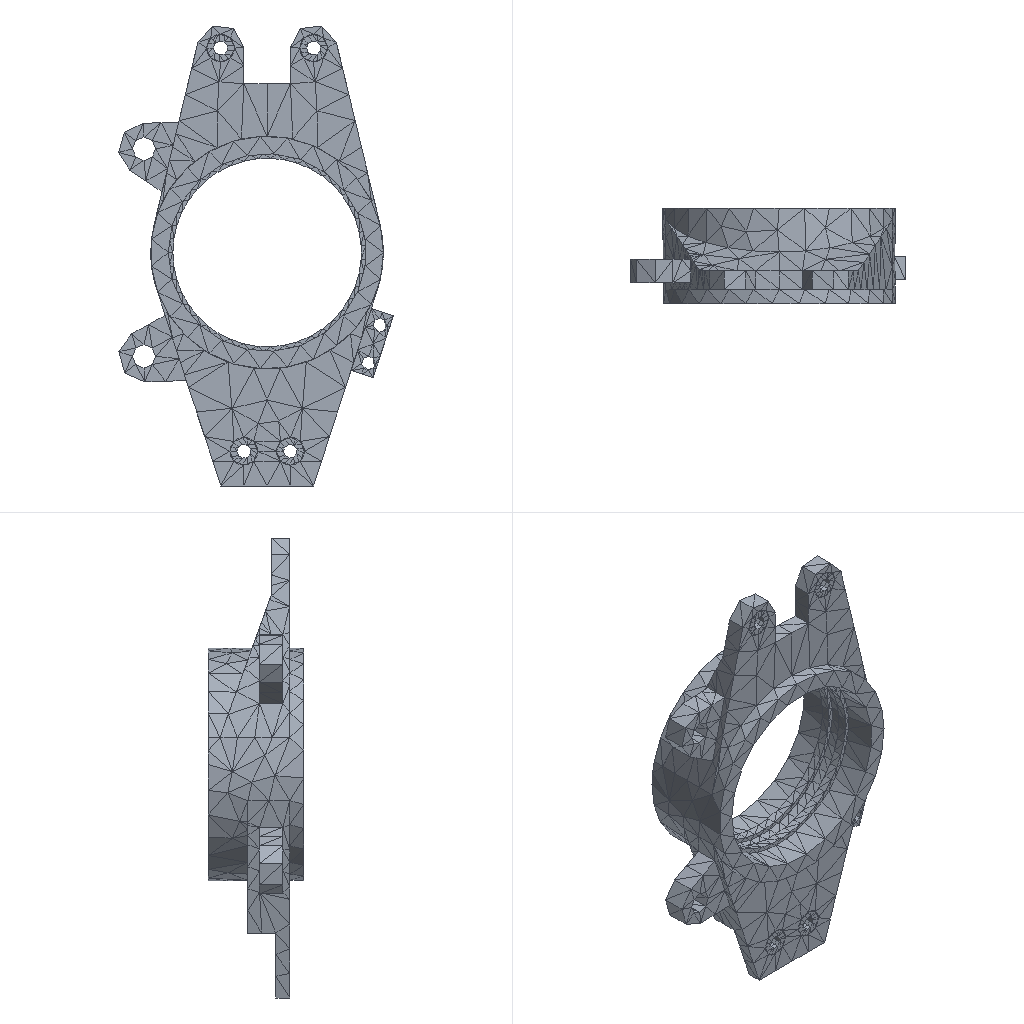Simulation study | ansys workbench
Ansys APDL input file, long lists of numbers shortened:
/batch
/config,noeldb,1     ! force off writing results to database
*get,_wallstrt,active,,time,wall
! ANSYS input file written by Workbench version 2022 R1
! File used for geometry attach:
/title,__1--____ (B5)
! ****** Begin Custom Load Command Snippet ******
/COM, ACT Extensions:
/COM,     LSDYNA, 2021.1
/COM,
! ****** End   Custom Load Command Snippet ******
*DIM,_wb_ProjectScratch_dir,string,248
_wb_ProjectScratch_dir(1) = ''
*DIM,_wb_SolverFiles_dir,string,248
_wb_SolverFiles_dir(1) = ''
*DIM,_wb_userfiles_dir,string,248
_wb_userfiles_dir(1) = ''
/com,--- Data in consistent NMM units. See Solving Units in the help system for more information.
/units,MPA
/nopr
/wb,file,start              !  signify a WB generated input file
/prep7
! Turn off shape checking because checks already performed inside WB mesher.
! See help system for more information.
SHPP,OFF,,NOWARN
/nolist
etcon,set             ! allow ANSYS to choose best KEYOP's for 180x elements, resets any applicable keyopt to MAPDL defaults
/com,*********** Nodes for the whole assembly ***********
nblock,3,,8127
(1i9,3e20.9e3)
        1    -1.253072820E+01    -1.049943652E+01    -8.837560534E+01
! (7388 more lines like these left out)
-1
/wb,elem,start            !  set before creation of elements
/com,*********** Elements for Body 1 "SYS\fix_end 2" ***********
et,1,186
keyo,1,2,1          ! set full integration on SOLID186
eblock,19,solid,,76
(19i9)
        1        1        1        1        0        0        0        0       20        0      115      775      879      878      810      778      913      894      834
! (151 more lines like these left out)
-1
/com,*********** Elements for Body 2 "SYS\fix_end 3" ***********
et,2,186
keyo,2,2,1          ! set full integration on SOLID186
eblock,19,solid,,76
(19i9)
        2        2        2        2        0        0        0        0       20        0      191     1324     1348     1349     1325     1336     1404     1403     1337
! (151 more lines like these left out)
-1
/com,*********** Elements for Body 3 "SYS\fix_end 4" ***********
et,3,186
keyo,3,2,1          ! set full integration on SOLID186
eblock,19,solid,,57
(19i9)
        3        3        3        3        0        0        0        0       20        0        1       45       68       69       46       60      103      104       59
! (113 more lines like these left out)
-1
/com,*********** Elements for Body 4 "SYS\fix_end 1" ***********
et,4,186
keyo,4,2,1          ! set full integration on SOLID186
eblock,19,solid,,57
(19i9)
        4        4        4        4        0        0        0        0       20        0       58      429      452      453      430      444      487      488      443
! (113 more lines like these left out)
-1
/com,*********** Elements for Body 5 "SYS\qianzhuan" ***********
et,5,187
eblock,19,solid,,2770
(19i9)
        5        5        5        5        0        0        0        0       10        0      267     1940     1947     1957     2732     3818     3885     3819     3821
! (5539 more lines like these left out)
-1
/wb,elem,end               !  done creating elements
/com,*********** Send User Defined Coordinate System(s) ***********
csys,0
toffst,273.15,  ! Temperature offset from absolute zero
/com,*********** Set Reference Temperature ***********
tref,22.
/wb,mat,start              !  starting to send materials
/com,*********** Send Materials ***********
MP,EX,1,68950,	! tonne s^-2 mm^-1
MP,NUXY,1,0.33,
MP,DENS,1,2.7e-09,	! tonne mm^-3
MP,ALPX,1,7.88860905221012e-31,	! C^-1
! (31 more lines like these left out)
/wb,mat,end                !  done sending materials
!************************* Model Summary ********************
!SYS\fix_end 2,	Aluminum 6061-T6; 6061-T651,	matid,	1
!SYS\fix_end 3,	Aluminum 6061-T6; 6061-T651,	matid,	2
!SYS\fix_end 4,	Aluminum 6061-T6; 6061-T651,	matid,	3
!SYS\fix_end 1,	Aluminum 6061-T6; 6061-T651,	matid,	4
!SYS\qianzhuan,	Aluminum 6061-T6; 6061-T651,	matid,	5
!************************* End Model Summary ********************
! get the diagonal of the bounding box. Needed later for other things
*get,_xmin,node,,mnloc,x
*get,_ymin,node,,mnloc,y
*get,_zmin,node,,mnloc,z
*get,_xmax,node,,mxloc,x
*get,_ymax,node,,mxloc,y
*get,_zmax,node,,mxloc,z
_ASMDIAG=(_xmax-_xmin)*(_xmax-_xmin)+(_ymax-_ymin)*(_ymax-_ymin)+(_zmax-_zmin)*(_zmax-_zmin)
_ASMDIAG=SQRT(_ASMDIAG)
/wb,contact,start          !  starting to send contact
/com,*********** Create Contact "接触区域" ***********
/com,            Real Constant Set For Above Contact Is 7 & 6
*set,tid,7
*set,cid,6
r,tid
r,cid
et,tid,170
et,cid,174
eblock,10,,,68
(15i9)
     5355        7        7        7        0      799      784      895      846      962      964     1153     1008
! (67 more lines like these left out)
-1
eblock,10,,,68
(15i9)
     5423        6        6        6        0      799      784      895      846      962      964     1153     1008
! (67 more lines like these left out)
-1
eblock,10,,,16
(15i9)
     5491        6        7        6        0     1806     1809     1820     1820     2991     3013     1820     2995
! (15 more lines like these left out)
-1
eblock,10,,,16
(15i9)
     5507        7        6        7        0     1806     1809     1820     1820     2991     3013     1820     2995
! (15 more lines like these left out)
-1
keyo,cid,8,2               ! auto create asymmetric contact (from Program Controlled setting)
keyo,cid,10,0              ! adjust contact stiffness each NR iteration (from Program Controlled setting)
keyo,cid,12,5              ! bonded always
keyo,cid,18,1              ! small sliding turned on by application
keyo,cid,2,0               ! augmented Lagrange (from Program Controlled setting)
keyo,cid,4,0               ! on Gauss point (from Program Controlled setting)
keyo,cid,9,1               ! ignore initial gaps/penetration
keyo,cid,7,0               ! No Prediction
rmod,tid,3,10.      ! FKN
rmod,tid,5,0.       ! ICONT
rmod,tid,6,0.       ! PINB
rmod,tid,10,0.      ! CNOF
rmod,tid,12,0.      ! FKT
rmod,tid,36,39      ! WB DSID
rmod,cid,3,10.      ! FKN
rmod,cid,5,0.       ! ICONT
rmod,cid,6,0.       ! PINB
rmod,cid,10,0.      ! CNOF
rmod,cid,12,0.      ! FKT
rmod,cid,36,39      ! WB DSID
/com,*********** Create Contact "接触区域 2" ***********
/com,            Real Constant Set For Above Contact Is 9 & 8
*set,tid,9
*set,cid,8
r,tid
r,cid
et,tid,170
et,cid,174
eblock,10,,,68
(15i9)
     5523        9        9        9        0     1390     1391     1392     1342     1737     1739     1641     1640
! (67 more lines like these left out)
-1
eblock,10,,,68
(15i9)
     5591        8        8        8        0     1390     1391     1392     1342     1737     1739     1641     1640
! (67 more lines like these left out)
-1
eblock,10,,,16
(15i9)
     5659        8        9        8        0     1790     1793     1800     1800     2910     2930     1800     2912
! (15 more lines like these left out)
-1
eblock,10,,,16
(15i9)
     5675        9        8        9        0     1790     1793     1800     1800     2910     2930     1800     2912
! (15 more lines like these left out)
-1
keyo,cid,8,2               ! auto create asymmetric contact (from Program Controlled setting)
keyo,cid,10,0              ! adjust contact stiffness each NR iteration (from Program Controlled setting)
keyo,cid,12,5              ! bonded always
keyo,cid,18,1              ! small sliding turned on by application
keyo,cid,2,0               ! augmented Lagrange (from Program Controlled setting)
keyo,cid,4,0               ! on Gauss point (from Program Controlled setting)
keyo,cid,9,1               ! ignore initial gaps/penetration
keyo,cid,7,0               ! No Prediction
rmod,tid,3,10.      ! FKN
rmod,tid,5,0.       ! ICONT
rmod,tid,6,0.       ! PINB
rmod,tid,10,0.      ! CNOF
rmod,tid,12,0.      ! FKT
rmod,tid,36,42      ! WB DSID
rmod,cid,3,10.      ! FKN
rmod,cid,5,0.       ! ICONT
rmod,cid,6,0.       ! PINB
rmod,cid,10,0.      ! CNOF
rmod,cid,12,0.      ! FKT
rmod,cid,36,42      ! WB DSID
/com,*********** Create Contact "接触区域 3" ***********
/com,            Real Constant Set For Above Contact Is 11 & 10
*set,tid,11
*set,cid,10
r,tid
r,cid
et,tid,170
et,cid,174
eblock,10,,,51
(15i9)
     5691       11       11       11        0       94       95       96       62      366      368      303      302
! (50 more lines like these left out)
-1
eblock,10,,,51
(15i9)
     5742       10       10       10        0       94       95       96       62      366      368      303      302
! (50 more lines like these left out)
-1
eblock,10,,,16
(15i9)
     5793       10       11       10        0     1779     1775     1786     1786     2839     2841     1786     2861
! (15 more lines like these left out)
-1
eblock,10,,,16
(15i9)
     5809       11       10       11        0     1779     1775     1786     1786     2839     2841     1786     2861
! (15 more lines like these left out)
-1
keyo,cid,8,2               ! auto create asymmetric contact (from Program Controlled setting)
keyo,cid,10,0              ! adjust contact stiffness each NR iteration (from Program Controlled setting)
keyo,cid,12,5              ! bonded always
keyo,cid,18,1              ! small sliding turned on by application
keyo,cid,2,0               ! augmented Lagrange (from Program Controlled setting)
keyo,cid,4,0               ! on Gauss point (from Program Controlled setting)
keyo,cid,9,1               ! ignore initial gaps/penetration
keyo,cid,7,0               ! No Prediction
rmod,tid,3,10.      ! FKN
rmod,tid,5,0.       ! ICONT
rmod,tid,6,0.       ! PINB
rmod,tid,10,0.      ! CNOF
rmod,tid,12,0.      ! FKT
rmod,tid,36,45      ! WB DSID
rmod,cid,3,10.      ! FKN
rmod,cid,5,0.       ! ICONT
rmod,cid,6,0.       ! PINB
rmod,cid,10,0.      ! CNOF
rmod,cid,12,0.      ! FKT
rmod,cid,36,45      ! WB DSID
/com,*********** Create Contact "接触区域 4" ***********
/com,            Real Constant Set For Above Contact Is 13 & 12
*set,tid,13
*set,cid,12
r,tid
r,cid
et,tid,170
et,cid,174
eblock,10,,,51
(15i9)
     5825       13       13       13        0      478      479      480      446      750      752      687      686
! (50 more lines like these left out)
-1
eblock,10,,,51
(15i9)
     5876       12       12       12        0      478      479      480      446      750      752      687      686
! (50 more lines like these left out)
-1
eblock,10,,,16
(15i9)
     5927       12       13       12        0     1761     1765     1772     1772     2763     2793     1772     2765
! (15 more lines like these left out)
-1
eblock,10,,,16
(15i9)
     5943       13       12       13        0     1761     1765     1772     1772     2763     2793     1772     2765
! (15 more lines like these left out)
-1
keyo,cid,8,2               ! auto create asymmetric contact (from Program Controlled setting)
keyo,cid,10,0              ! adjust contact stiffness each NR iteration (from Program Controlled setting)
keyo,cid,12,5              ! bonded always
keyo,cid,18,1              ! small sliding turned on by application
keyo,cid,2,0               ! augmented Lagrange (from Program Controlled setting)
keyo,cid,4,0               ! on Gauss point (from Program Controlled setting)
keyo,cid,9,1               ! ignore initial gaps/penetration
keyo,cid,7,0               ! No Prediction
rmod,tid,3,10.      ! FKN
rmod,tid,5,0.       ! ICONT
rmod,tid,6,0.       ! PINB
rmod,tid,10,0.      ! CNOF
rmod,tid,12,0.      ! FKT
rmod,tid,36,48      ! WB DSID
rmod,cid,3,10.      ! FKN
rmod,cid,5,0.       ! ICONT
rmod,cid,6,0.       ! PINB
rmod,cid,10,0.      ! CNOF
rmod,cid,12,0.      ! FKT
rmod,cid,36,48      ! WB DSID
nsel,all
esel,all
/wb,contact,end            !  done creating contacts
/golist
/wb,load,start             !  starting to send loads
/com,*********** Fixed Supports ***********
CMBLOCK,_FIXEDSU,NODE,      544
(8i10)
        26        27        28        29        30        31        32        33
! (67 more lines like these left out)
cmsel,s,_FIXEDSU
d,all,all
nsel,all
/com,*********** Define Line Pressure Vector Using Surface Effect Elements ***********
local,12,0,0.,0.,0.,0.,0.,0.
csys,0
et,14,156
keyop,14,5,1        !  No orientation node
eblock,10,,,123
(15i9)
     5959       14       14       14       12     2522     2523     6960
! (122 more lines like these left out)
-1
esel,s,type,,14
keyop,14,2,1                ! Apply load in local coordinate system
esel,all
/gst,on,on
fini
*get,_numnode,node,0,count
*get,_numelem,elem,0,count
*get, _MAXELEMNUM, elem, 0, NUM, MAX
*get, _MAXNODENUM, node, 0, NUM, MAX
*get, _MAXELEMTYPE, etyp, 0, NUM, MAX
*get, _MAXREALCONST, real, 0, NUM, MAX
/go
/wb,load,end               !  done creating loads
/com,--- Number of total nodes = %_numnode%
/com,--- Number of contact elements = 727
/com,--- Number of spring elements = 0
/com,--- Number of bearing elements = 0
/com,--- Number of solid elements = 3036
/com,--- Number of condensed parts = 0
/com,--- Number of total elements = %_numelem%
*get,_wallbsol,active,,time,wall
/com,****************************************************************************
/com,*************************    SOLUTION       ********************************
/com,****************************************************************************
/solu
antype,0                   ! static analysis
_thickRatio=0.2     ! Ratio of thick parts in the model
eqsl,sparse,,,,,1
cntr,print,1               ! print out contact info and also make no initial contact an error
dmpoption,emat,no             ! Don't combine emat file for DANSYS
dmpoption,esav,no             ! Don't combine esav file for DANSYS
nldiag,cont,iter           ! print out contact info each equilibrium iteration
rescontrol,,none                 ! Do not keep any restart files
/com,****************************************************
/com,******************* SOLVE FOR LS 1 OF 1 ****************
esel,s,type,,14
nsle
sfe,all,1,pres,1,318.
sfe,all,2,pres,1,0.
sfe,all,3,pres,1,0.
nsel,all
esel,all
/nopr
/gopr
nsub,1,1,1
time,1.
outres,erase
outres,all,none
outres,nsol,all,
outres,rsol,all
outres,eangl,all
outres,etmp,all
outres,veng,all
outres,strs,all,
outres,epel,all,
outres,eppl,all,
outres,cont,all,
! *********** WB SOLVE COMMAND ***********
! check interactive state
*get,ANSINTER_,active,,int
*if,ANSINTER_,ne,0,then
/eof
*endif
solve
/com *************** Write FE CONNECTORS *********
CEWRITE,file,ce,,INTE
/com,****************************************************
/com,*************** FINISHED SOLVE FOR LS 1 *************
*get,_wallasol,active,,time,wall
/nopr
*get,_numnode,node,0,count
*get,_numelem,elem,0,count
*get, _MAXELEMNUM, elem, 0, NUM, MAX
*get, _MAXNODENUM, node, 0, NUM, MAX,,,INTERNAL
*get, _MAXELEMTYPE, etyp, 0, NUM, MAX
*get, _MAXREALCONST, real, 0, NUM, MAX
/gopr
/post1
xmlo,ENCODING,ISO-8859-1
xmlo,parm
/xml,parm,xml
fini
/gopr
*get,_walldone,active,,time,wall
_preptime=(_wallbsol-_wallstrt)*3600
_solvtime=(_wallasol-_wallbsol)*3600
_posttime=(_walldone-_wallasol)*3600
_totaltim=(_walldone-_wallstrt)*3600
*get,_dlbratio,active,0,solu,dlbr
*get,_combtime,active,0,solu,comb
*get,_ssmode,active,0,solu,ssmm
*get,_ndofs,active,0,solu,ndof
*get,_sol_end_time,active,0,set,time
*if,_sol_end_time,eq,1.,then
/fclean				!clean distributed files
*endif
/com,--- Total number of nodes = %_numnode%
/com,--- Total number of elements = %_numelem%
/com,--- Element load balance ratio = %_dlbratio%
/com,--- Time to combine distributed files = %_combtime%
/com,--- Sparse memory mode = %_ssmode%
/com,--- Number of DOF = %_ndofs%
/wb,file,end               ! done with WB generated input